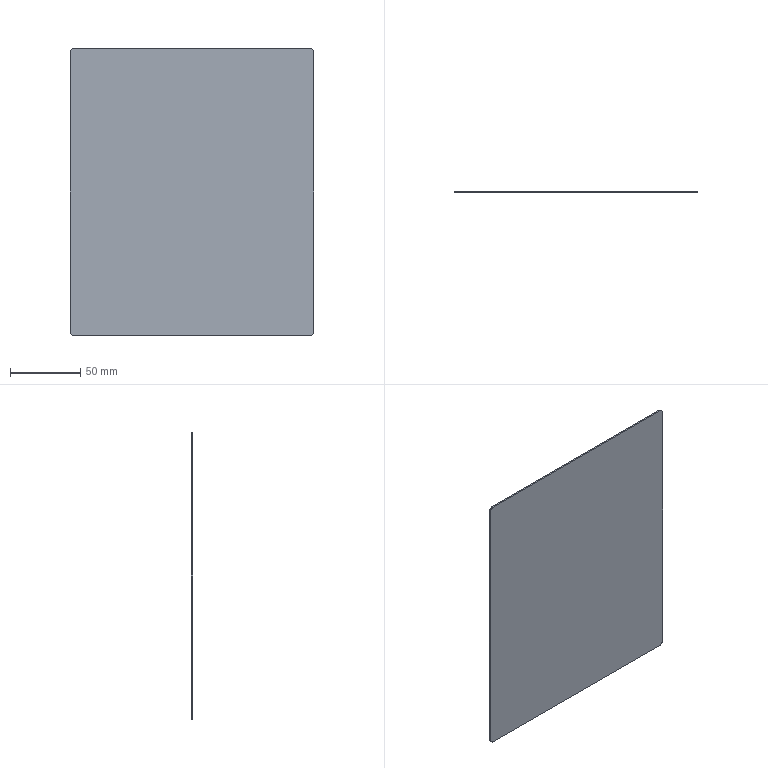Part | NX | features BREP 1 | 1 solid | 10 faces | box 173 x 1 x 204 mm | volume 35284 mm3 | plane 6 | cylinder 4 | commonest cylinder face diameters 6 x4
STEP:
#1=CARTESIAN_POINT('',(-86.5,1.,99.));
#2=VERTEX_POINT('',#1);
#3=CARTESIAN_POINT('',(-83.5,1.,102.));
#4=VERTEX_POINT('',#3);
#5=CARTESIAN_POINT('',(-83.5,1.,99.));
#6=DIRECTION('',(0.,1.,0.));
#7=DIRECTION('',(0.,0.,-1.));
#8=AXIS2_PLACEMENT_3D('',#5,#6,#7);
#9=CIRCLE('',#8,3.);
#10=EDGE_CURVE('',#2,#4,#9,.T.);
#11=ORIENTED_EDGE('',*,*,#10,.T.);
#12=CARTESIAN_POINT('',(83.5,1.,102.));
#13=VERTEX_POINT('',#12);
#14=CARTESIAN_POINT('',(0.,1.,102.));
#15=DIRECTION('',(1.,0.,0.));
#16=VECTOR('',#15,1000.);
#17=LINE('',#14,#16);
#18=EDGE_CURVE('',#4,#13,#17,.T.);
#19=ORIENTED_EDGE('',*,*,#18,.T.);
#20=CARTESIAN_POINT('',(86.5,1.,99.));
#21=VERTEX_POINT('',#20);
#22=CARTESIAN_POINT('',(83.5,1.,99.));
#23=DIRECTION('',(0.,1.,0.));
#24=DIRECTION('',(0.,0.,-1.));
#25=AXIS2_PLACEMENT_3D('',#22,#23,#24);
#26=CIRCLE('',#25,3.);
#27=EDGE_CURVE('',#13,#21,#26,.T.);
#28=ORIENTED_EDGE('',*,*,#27,.T.);
#29=CARTESIAN_POINT('',(86.5,1.,-99.));
#30=VERTEX_POINT('',#29);
#31=CARTESIAN_POINT('',(86.5,1.,0.));
#32=DIRECTION('',(0.,0.,-1.));
#33=VECTOR('',#32,1000.);
#34=LINE('',#31,#33);
#35=EDGE_CURVE('',#21,#30,#34,.T.);
#36=ORIENTED_EDGE('',*,*,#35,.T.);
#37=CARTESIAN_POINT('',(83.5,1.,-102.));
#38=VERTEX_POINT('',#37);
#39=CARTESIAN_POINT('',(83.5,1.,-99.));
#40=DIRECTION('',(0.,1.,0.));
#41=DIRECTION('',(0.,0.,-1.));
#42=AXIS2_PLACEMENT_3D('',#39,#40,#41);
#43=CIRCLE('',#42,3.);
#44=EDGE_CURVE('',#30,#38,#43,.T.);
#45=ORIENTED_EDGE('',*,*,#44,.T.);
#46=CARTESIAN_POINT('',(-83.5,1.,-102.));
#47=VERTEX_POINT('',#46);
#48=CARTESIAN_POINT('',(0.,1.,-102.));
#49=DIRECTION('',(-1.,0.,0.));
#50=VECTOR('',#49,1000.);
#51=LINE('',#48,#50);
#52=EDGE_CURVE('',#38,#47,#51,.T.);
#53=ORIENTED_EDGE('',*,*,#52,.T.);
#54=CARTESIAN_POINT('',(-86.5,1.,-99.));
#55=VERTEX_POINT('',#54);
#56=CARTESIAN_POINT('',(-83.5,1.,-99.));
#57=DIRECTION('',(0.,1.,0.));
#58=DIRECTION('',(0.,0.,-1.));
#59=AXIS2_PLACEMENT_3D('',#56,#57,#58);
#60=CIRCLE('',#59,3.);
#61=EDGE_CURVE('',#47,#55,#60,.T.);
#62=ORIENTED_EDGE('',*,*,#61,.T.);
#63=CARTESIAN_POINT('',(-86.5,1.,0.));
#64=DIRECTION('',(0.,0.,1.));
#65=VECTOR('',#64,1000.);
#66=LINE('',#63,#65);
#67=EDGE_CURVE('',#55,#2,#66,.T.);
#68=ORIENTED_EDGE('',*,*,#67,.T.);
#69=EDGE_LOOP('',(#11,#19,#28,#36,#45,#53,#62,#68));
#70=FACE_BOUND('',#69,.T.);
#71=CARTESIAN_POINT('',(0.,1.,0.));
#72=DIRECTION('',(0.,1.,0.));
#73=DIRECTION('',(0.,0.,-1.));
#74=AXIS2_PLACEMENT_3D('',#71,#72,#73);
#75=PLANE('',#74);
#76=ADVANCED_FACE('',(#70),#75,.T.);
#77=CARTESIAN_POINT('',(83.5,0.,102.));
#78=VERTEX_POINT('',#77);
#79=CARTESIAN_POINT('',(83.5,0.,102.));
#80=DIRECTION('',(0.,1.,0.));
#81=VECTOR('',#80,1000.);
#82=LINE('',#79,#81);
#83=EDGE_CURVE('',#78,#13,#82,.T.);
#84=ORIENTED_EDGE('',*,*,#83,.T.);
#85=ORIENTED_EDGE('',*,*,#18,.F.);
#86=CARTESIAN_POINT('',(-83.5,0.,102.));
#87=VERTEX_POINT('',#86);
#88=CARTESIAN_POINT('',(-83.5,0.,102.));
#89=DIRECTION('',(0.,-1.,0.));
#90=VECTOR('',#89,1000.);
#91=LINE('',#88,#90);
#92=EDGE_CURVE('',#4,#87,#91,.T.);
#93=ORIENTED_EDGE('',*,*,#92,.T.);
#94=CARTESIAN_POINT('',(-86.5,0.,102.));
#95=DIRECTION('',(1.,0.,0.));
#96=VECTOR('',#95,1000.);
#97=LINE('',#94,#96);
#98=EDGE_CURVE('',#87,#78,#97,.T.);
#99=ORIENTED_EDGE('',*,*,#98,.T.);
#100=EDGE_LOOP('',(#84,#85,#93,#99));
#101=FACE_BOUND('',#100,.T.);
#102=CARTESIAN_POINT('',(-86.5,0.,102.));
#103=DIRECTION('',(0.,0.,1.));
#104=DIRECTION('',(-1.,0.,0.));
#105=AXIS2_PLACEMENT_3D('',#102,#103,#104);
#106=PLANE('',#105);
#107=ADVANCED_FACE('',(#101),#106,.T.);
#108=ORIENTED_EDGE('',*,*,#92,.F.);
#109=ORIENTED_EDGE('',*,*,#10,.F.);
#110=CARTESIAN_POINT('',(-86.5,0.,99.));
#111=VERTEX_POINT('',#110);
#112=CARTESIAN_POINT('',(-86.5,4.158,99.));
#113=DIRECTION('',(0.,-1.,0.));
#114=VECTOR('',#113,1000.);
#115=LINE('',#112,#114);
#116=EDGE_CURVE('',#2,#111,#115,.T.);
#117=ORIENTED_EDGE('',*,*,#116,.T.);
#118=CARTESIAN_POINT('',(-83.5,0.,99.));
#119=DIRECTION('',(0.,1.,0.));
#120=DIRECTION('',(0.,0.,-1.));
#121=AXIS2_PLACEMENT_3D('',#118,#119,#120);
#122=CIRCLE('',#121,3.);
#123=EDGE_CURVE('',#111,#87,#122,.T.);
#124=ORIENTED_EDGE('',*,*,#123,.T.);
#125=EDGE_LOOP('',(#108,#109,#117,#124));
#126=FACE_BOUND('',#125,.T.);
#127=CARTESIAN_POINT('',(-83.5,4.158,99.));
#128=DIRECTION('',(0.,-1.,0.));
#129=DIRECTION('',(0.,0.,1.));
#130=AXIS2_PLACEMENT_3D('',#127,#128,#129);
#131=CYLINDRICAL_SURFACE('',#130,3.);
#132=ADVANCED_FACE('',(#126),#131,.T.);
#133=ORIENTED_EDGE('',*,*,#116,.F.);
#134=ORIENTED_EDGE('',*,*,#67,.F.);
#135=CARTESIAN_POINT('',(-86.5,0.,-99.));
#136=VERTEX_POINT('',#135);
#137=CARTESIAN_POINT('',(-86.5,0.,-99.));
#138=DIRECTION('',(0.,-1.,0.));
#139=VECTOR('',#138,1000.);
#140=LINE('',#137,#139);
#141=EDGE_CURVE('',#55,#136,#140,.T.);
#142=ORIENTED_EDGE('',*,*,#141,.T.);
#143=CARTESIAN_POINT('',(-86.5,0.,-102.));
#144=DIRECTION('',(0.,0.,1.));
#145=VECTOR('',#144,1000.);
#146=LINE('',#143,#145);
#147=EDGE_CURVE('',#136,#111,#146,.T.);
#148=ORIENTED_EDGE('',*,*,#147,.T.);
#149=EDGE_LOOP('',(#133,#134,#142,#148));
#150=FACE_BOUND('',#149,.T.);
#151=CARTESIAN_POINT('',(-86.5,0.,-102.));
#152=DIRECTION('',(-1.,0.,0.));
#153=DIRECTION('',(0.,0.,-1.));
#154=AXIS2_PLACEMENT_3D('',#151,#152,#153);
#155=PLANE('',#154);
#156=ADVANCED_FACE('',(#150),#155,.T.);
#157=CARTESIAN_POINT('',(-83.5,0.,-102.));
#158=VERTEX_POINT('',#157);
#159=CARTESIAN_POINT('',(-83.5,4.158,-102.));
#160=DIRECTION('',(0.,-1.,0.));
#161=VECTOR('',#160,1000.);
#162=LINE('',#159,#161);
#163=EDGE_CURVE('',#47,#158,#162,.T.);
#164=ORIENTED_EDGE('',*,*,#163,.T.);
#165=CARTESIAN_POINT('',(-83.5,0.,-99.));
#166=DIRECTION('',(0.,1.,0.));
#167=DIRECTION('',(0.,0.,-1.));
#168=AXIS2_PLACEMENT_3D('',#165,#166,#167);
#169=CIRCLE('',#168,3.);
#170=EDGE_CURVE('',#158,#136,#169,.T.);
#171=ORIENTED_EDGE('',*,*,#170,.T.);
#172=ORIENTED_EDGE('',*,*,#141,.F.);
#173=ORIENTED_EDGE('',*,*,#61,.F.);
#174=EDGE_LOOP('',(#164,#171,#172,#173));
#175=FACE_BOUND('',#174,.T.);
#176=CARTESIAN_POINT('',(-83.5,4.158,-99.));
#177=DIRECTION('',(0.,-1.,0.));
#178=DIRECTION('',(0.,0.,1.));
#179=AXIS2_PLACEMENT_3D('',#176,#177,#178);
#180=CYLINDRICAL_SURFACE('',#179,3.);
#181=ADVANCED_FACE('',(#175),#180,.T.);
#182=CARTESIAN_POINT('',(83.5,0.,-102.));
#183=VERTEX_POINT('',#182);
#184=CARTESIAN_POINT('',(83.5,0.,-102.));
#185=DIRECTION('',(0.,-1.,0.));
#186=VECTOR('',#185,1000.);
#187=LINE('',#184,#186);
#188=EDGE_CURVE('',#38,#183,#187,.T.);
#189=ORIENTED_EDGE('',*,*,#188,.T.);
#190=CARTESIAN_POINT('',(86.5,0.,-102.));
#191=DIRECTION('',(-1.,0.,0.));
#192=VECTOR('',#191,1000.);
#193=LINE('',#190,#192);
#194=EDGE_CURVE('',#183,#158,#193,.T.);
#195=ORIENTED_EDGE('',*,*,#194,.T.);
#196=ORIENTED_EDGE('',*,*,#163,.F.);
#197=ORIENTED_EDGE('',*,*,#52,.F.);
#198=EDGE_LOOP('',(#189,#195,#196,#197));
#199=FACE_BOUND('',#198,.T.);
#200=CARTESIAN_POINT('',(86.5,0.,-102.));
#201=DIRECTION('',(0.,0.,-1.));
#202=DIRECTION('',(1.,0.,0.));
#203=AXIS2_PLACEMENT_3D('',#200,#201,#202);
#204=PLANE('',#203);
#205=ADVANCED_FACE('',(#199),#204,.T.);
#206=CARTESIAN_POINT('',(86.5,0.,-99.));
#207=VERTEX_POINT('',#206);
#208=CARTESIAN_POINT('',(86.5,4.158,-99.));
#209=DIRECTION('',(0.,-1.,0.));
#210=VECTOR('',#209,1000.);
#211=LINE('',#208,#210);
#212=EDGE_CURVE('',#30,#207,#211,.T.);
#213=ORIENTED_EDGE('',*,*,#212,.T.);
#214=CARTESIAN_POINT('',(83.5,0.,-99.));
#215=DIRECTION('',(0.,1.,0.));
#216=DIRECTION('',(0.,0.,-1.));
#217=AXIS2_PLACEMENT_3D('',#214,#215,#216);
#218=CIRCLE('',#217,3.);
#219=EDGE_CURVE('',#207,#183,#218,.T.);
#220=ORIENTED_EDGE('',*,*,#219,.T.);
#221=ORIENTED_EDGE('',*,*,#188,.F.);
#222=ORIENTED_EDGE('',*,*,#44,.F.);
#223=EDGE_LOOP('',(#213,#220,#221,#222));
#224=FACE_BOUND('',#223,.T.);
#225=CARTESIAN_POINT('',(83.5,4.158,-99.));
#226=DIRECTION('',(0.,-1.,0.));
#227=DIRECTION('',(0.,0.,1.));
#228=AXIS2_PLACEMENT_3D('',#225,#226,#227);
#229=CYLINDRICAL_SURFACE('',#228,3.);
#230=ADVANCED_FACE('',(#224),#229,.T.);
#231=ORIENTED_EDGE('',*,*,#212,.F.);
#232=ORIENTED_EDGE('',*,*,#35,.F.);
#233=CARTESIAN_POINT('',(86.5,0.,99.));
#234=VERTEX_POINT('',#233);
#235=CARTESIAN_POINT('',(86.5,0.,99.));
#236=DIRECTION('',(0.,-1.,0.));
#237=VECTOR('',#236,1000.);
#238=LINE('',#235,#237);
#239=EDGE_CURVE('',#21,#234,#238,.T.);
#240=ORIENTED_EDGE('',*,*,#239,.T.);
#241=CARTESIAN_POINT('',(86.5,0.,102.));
#242=DIRECTION('',(0.,0.,-1.));
#243=VECTOR('',#242,1000.);
#244=LINE('',#241,#243);
#245=EDGE_CURVE('',#234,#207,#244,.T.);
#246=ORIENTED_EDGE('',*,*,#245,.T.);
#247=EDGE_LOOP('',(#231,#232,#240,#246));
#248=FACE_BOUND('',#247,.T.);
#249=CARTESIAN_POINT('',(86.5,0.,102.));
#250=DIRECTION('',(1.,0.,0.));
#251=DIRECTION('',(0.,0.,1.));
#252=AXIS2_PLACEMENT_3D('',#249,#250,#251);
#253=PLANE('',#252);
#254=ADVANCED_FACE('',(#248),#253,.T.);
#255=ORIENTED_EDGE('',*,*,#239,.F.);
#256=ORIENTED_EDGE('',*,*,#27,.F.);
#257=ORIENTED_EDGE('',*,*,#83,.F.);
#258=CARTESIAN_POINT('',(83.5,0.,99.));
#259=DIRECTION('',(0.,1.,0.));
#260=DIRECTION('',(0.,0.,-1.));
#261=AXIS2_PLACEMENT_3D('',#258,#259,#260);
#262=CIRCLE('',#261,3.);
#263=EDGE_CURVE('',#78,#234,#262,.T.);
#264=ORIENTED_EDGE('',*,*,#263,.T.);
#265=EDGE_LOOP('',(#255,#256,#257,#264));
#266=FACE_BOUND('',#265,.T.);
#267=CARTESIAN_POINT('',(83.5,4.158,99.));
#268=DIRECTION('',(0.,-1.,0.));
#269=DIRECTION('',(0.,0.,1.));
#270=AXIS2_PLACEMENT_3D('',#267,#268,#269);
#271=CYLINDRICAL_SURFACE('',#270,3.);
#272=ADVANCED_FACE('',(#266),#271,.T.);
#273=ORIENTED_EDGE('',*,*,#245,.F.);
#274=ORIENTED_EDGE('',*,*,#263,.F.);
#275=ORIENTED_EDGE('',*,*,#98,.F.);
#276=ORIENTED_EDGE('',*,*,#123,.F.);
#277=ORIENTED_EDGE('',*,*,#147,.F.);
#278=ORIENTED_EDGE('',*,*,#170,.F.);
#279=ORIENTED_EDGE('',*,*,#194,.F.);
#280=ORIENTED_EDGE('',*,*,#219,.F.);
#281=EDGE_LOOP('',(#273,#274,#275,#276,#277,#278,#279,#280));
#282=FACE_BOUND('',#281,.T.);
#283=CARTESIAN_POINT('',(0.,0.,0.));
#284=DIRECTION('',(0.,1.,0.));
#285=DIRECTION('',(0.,0.,-1.));
#286=AXIS2_PLACEMENT_3D('',#283,#284,#285);
#287=PLANE('',#286);
#288=ADVANCED_FACE('',(#282),#287,.F.);
#289=CLOSED_SHELL('',(#76,#107,#132,#156,#181,#205,#230,#254,#272,#288));
#290=MANIFOLD_SOLID_BREP('',#289);
#291=(LENGTH_UNIT()NAMED_UNIT(*)SI_UNIT(.MILLI.,.METRE.));
#292=UNCERTAINTY_MEASURE_WITH_UNIT(LENGTH_MEASURE(0.00001),#291,'','');
#293=(NAMED_UNIT(*)PLANE_ANGLE_UNIT()SI_UNIT($,.RADIAN.));
#294=(NAMED_UNIT(*)SI_UNIT($,.STERADIAN.)SOLID_ANGLE_UNIT());
#295=(GEOMETRIC_REPRESENTATION_CONTEXT(3)GLOBAL_UNCERTAINTY_ASSIGNED_CONTEXT((#292))GLOBAL_UNIT_ASSIGNED_CONTEXT((#291,#293,#294))REPRESENTATION_CONTEXT('',''));
#296=ADVANCED_BREP_SHAPE_REPRESENTATION('',(#290),#295);